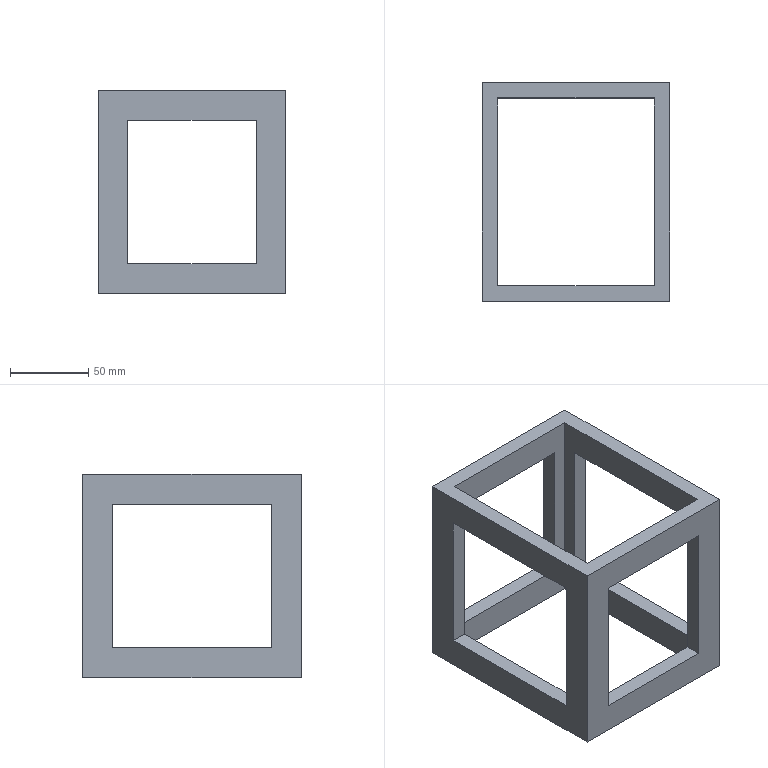Part | SolidWorks | features Cut 2, Extrusion 1 | 1 solid | 26 faces | box 119.912 x 140 x 130 mm | volume 285373 mm3 | plane 26
STEP:
#1=CARTESIAN_POINT('',(-70.,109.,-111.));
#2=VERTEX_POINT('',#1);
#3=CARTESIAN_POINT('',(-70.,109.,-19.));
#4=VERTEX_POINT('',#3);
#5=CARTESIAN_POINT('',(-70.,109.,-111.));
#6=DIRECTION('',(0.,0.,1.));
#7=VECTOR('',#6,1000.);
#8=LINE('',#5,#7);
#9=EDGE_CURVE('',#2,#4,#8,.T.);
#10=ORIENTED_EDGE('',*,*,#9,.F.);
#11=CARTESIAN_POINT('',(-70.,211.,-111.));
#12=VERTEX_POINT('',#11);
#13=CARTESIAN_POINT('',(-70.,211.,-111.));
#14=DIRECTION('',(0.,-1.,0.));
#15=VECTOR('',#14,1000.);
#16=LINE('',#13,#15);
#17=EDGE_CURVE('',#12,#2,#16,.T.);
#18=ORIENTED_EDGE('',*,*,#17,.F.);
#19=CARTESIAN_POINT('',(-70.,211.,-19.));
#20=VERTEX_POINT('',#19);
#21=CARTESIAN_POINT('',(-70.,211.,-19.));
#22=DIRECTION('',(0.,0.,-1.));
#23=VECTOR('',#22,1000.);
#24=LINE('',#21,#23);
#25=EDGE_CURVE('',#20,#12,#24,.T.);
#26=ORIENTED_EDGE('',*,*,#25,.F.);
#27=CARTESIAN_POINT('',(-70.,109.,-19.));
#28=DIRECTION('',(0.,1.,0.));
#29=VECTOR('',#28,1000.);
#30=LINE('',#27,#29);
#31=EDGE_CURVE('',#4,#20,#30,.T.);
#32=ORIENTED_EDGE('',*,*,#31,.F.);
#33=EDGE_LOOP('',(#10,#18,#26,#32));
#34=FACE_BOUND('',#33,.T.);
#35=CARTESIAN_POINT('',(-70.,230.,0.));
#36=VERTEX_POINT('',#35);
#37=CARTESIAN_POINT('',(-70.,90.,0.));
#38=VERTEX_POINT('',#37);
#39=CARTESIAN_POINT('',(-70.,230.,0.));
#40=DIRECTION('',(0.,-1.,0.));
#41=VECTOR('',#40,1000.);
#42=LINE('',#39,#41);
#43=EDGE_CURVE('',#36,#38,#42,.T.);
#44=ORIENTED_EDGE('',*,*,#43,.F.);
#45=CARTESIAN_POINT('',(-70.,230.,-130.));
#46=VERTEX_POINT('',#45);
#47=CARTESIAN_POINT('',(-70.,230.,-130.));
#48=DIRECTION('',(0.,0.,1.));
#49=VECTOR('',#48,1000.);
#50=LINE('',#47,#49);
#51=EDGE_CURVE('',#46,#36,#50,.T.);
#52=ORIENTED_EDGE('',*,*,#51,.F.);
#53=CARTESIAN_POINT('',(-70.,90.,-130.));
#54=VERTEX_POINT('',#53);
#55=CARTESIAN_POINT('',(-70.,230.,-130.));
#56=DIRECTION('',(0.,-1.,0.));
#57=VECTOR('',#56,1000.);
#58=LINE('',#55,#57);
#59=EDGE_CURVE('',#46,#54,#58,.T.);
#60=ORIENTED_EDGE('',*,*,#59,.T.);
#61=CARTESIAN_POINT('',(-70.,90.,-130.));
#62=DIRECTION('',(0.,0.,1.));
#63=VECTOR('',#62,1000.);
#64=LINE('',#61,#63);
#65=EDGE_CURVE('',#54,#38,#64,.T.);
#66=ORIENTED_EDGE('',*,*,#65,.T.);
#67=EDGE_LOOP('',(#44,#52,#60,#66));
#68=FACE_OUTER_BOUND('',#67,.T.);
#69=CARTESIAN_POINT('',(-70.,230.,-130.));
#70=DIRECTION('',(-1.,0.,0.));
#71=DIRECTION('',(0.,-1.,0.));
#72=AXIS2_PLACEMENT_3D('',#69,#70,#71);
#73=PLANE('',#72);
#74=ADVANCED_FACE('',(#34,#68),#73,.T.);
#75=CARTESIAN_POINT('',(30.912,230.,-19.));
#76=VERTEX_POINT('',#75);
#77=CARTESIAN_POINT('',(30.912,230.,-111.));
#78=VERTEX_POINT('',#77);
#79=CARTESIAN_POINT('',(30.912,230.,-130.));
#80=DIRECTION('',(0.,0.,-1.));
#81=VECTOR('',#80,1000.);
#82=LINE('',#79,#81);
#83=EDGE_CURVE('',#76,#78,#82,.T.);
#84=ORIENTED_EDGE('',*,*,#83,.F.);
#85=CARTESIAN_POINT('',(-51.,230.,-19.));
#86=VERTEX_POINT('',#85);
#87=CARTESIAN_POINT('',(49.912,230.,-19.));
#88=DIRECTION('',(1.,0.,0.));
#89=VECTOR('',#88,1000.);
#90=LINE('',#87,#89);
#91=EDGE_CURVE('',#86,#76,#90,.T.);
#92=ORIENTED_EDGE('',*,*,#91,.F.);
#93=CARTESIAN_POINT('',(-51.,230.,-111.));
#94=VERTEX_POINT('',#93);
#95=CARTESIAN_POINT('',(-51.,230.,-130.));
#96=DIRECTION('',(0.,0.,1.));
#97=VECTOR('',#96,1000.);
#98=LINE('',#95,#97);
#99=EDGE_CURVE('',#94,#86,#98,.T.);
#100=ORIENTED_EDGE('',*,*,#99,.F.);
#101=CARTESIAN_POINT('',(49.912,230.,-111.));
#102=DIRECTION('',(-1.,0.,0.));
#103=VECTOR('',#102,1000.);
#104=LINE('',#101,#103);
#105=EDGE_CURVE('',#78,#94,#104,.T.);
#106=ORIENTED_EDGE('',*,*,#105,.F.);
#107=EDGE_LOOP('',(#84,#92,#100,#106));
#108=FACE_BOUND('',#107,.T.);
#109=CARTESIAN_POINT('',(49.912,230.,0.));
#110=VERTEX_POINT('',#109);
#111=CARTESIAN_POINT('',(49.912,230.,0.));
#112=DIRECTION('',(-1.,0.,0.));
#113=VECTOR('',#112,1000.);
#114=LINE('',#111,#113);
#115=EDGE_CURVE('',#110,#36,#114,.T.);
#116=ORIENTED_EDGE('',*,*,#115,.F.);
#117=CARTESIAN_POINT('',(49.912,230.,-130.));
#118=VERTEX_POINT('',#117);
#119=CARTESIAN_POINT('',(49.912,230.,-130.));
#120=DIRECTION('',(0.,0.,1.));
#121=VECTOR('',#120,1000.);
#122=LINE('',#119,#121);
#123=EDGE_CURVE('',#118,#110,#122,.T.);
#124=ORIENTED_EDGE('',*,*,#123,.F.);
#125=CARTESIAN_POINT('',(49.912,230.,-130.));
#126=DIRECTION('',(-1.,0.,0.));
#127=VECTOR('',#126,1000.);
#128=LINE('',#125,#127);
#129=EDGE_CURVE('',#118,#46,#128,.T.);
#130=ORIENTED_EDGE('',*,*,#129,.T.);
#131=ORIENTED_EDGE('',*,*,#51,.T.);
#132=EDGE_LOOP('',(#116,#124,#130,#131));
#133=FACE_OUTER_BOUND('',#132,.T.);
#134=CARTESIAN_POINT('',(49.912,230.,-130.));
#135=DIRECTION('',(0.,1.,0.));
#136=DIRECTION('',(-1.,0.,0.));
#137=AXIS2_PLACEMENT_3D('',#134,#135,#136);
#138=PLANE('',#137);
#139=ADVANCED_FACE('',(#108,#133),#138,.T.);
#140=CARTESIAN_POINT('',(49.912,109.,-19.));
#141=VERTEX_POINT('',#140);
#142=CARTESIAN_POINT('',(49.912,109.,-111.));
#143=VERTEX_POINT('',#142);
#144=CARTESIAN_POINT('',(49.912,109.,-130.));
#145=DIRECTION('',(0.,0.,-1.));
#146=VECTOR('',#145,1000.);
#147=LINE('',#144,#146);
#148=EDGE_CURVE('',#141,#143,#147,.T.);
#149=ORIENTED_EDGE('',*,*,#148,.F.);
#150=CARTESIAN_POINT('',(49.912,211.,-19.));
#151=VERTEX_POINT('',#150);
#152=CARTESIAN_POINT('',(49.912,90.,-19.));
#153=DIRECTION('',(0.,-1.,0.));
#154=VECTOR('',#153,1000.);
#155=LINE('',#152,#154);
#156=EDGE_CURVE('',#151,#141,#155,.T.);
#157=ORIENTED_EDGE('',*,*,#156,.F.);
#158=CARTESIAN_POINT('',(49.912,211.,-111.));
#159=VERTEX_POINT('',#158);
#160=CARTESIAN_POINT('',(49.912,211.,-130.));
#161=DIRECTION('',(0.,0.,1.));
#162=VECTOR('',#161,1000.);
#163=LINE('',#160,#162);
#164=EDGE_CURVE('',#159,#151,#163,.T.);
#165=ORIENTED_EDGE('',*,*,#164,.F.);
#166=CARTESIAN_POINT('',(49.912,90.,-111.));
#167=DIRECTION('',(0.,1.,0.));
#168=VECTOR('',#167,1000.);
#169=LINE('',#166,#168);
#170=EDGE_CURVE('',#143,#159,#169,.T.);
#171=ORIENTED_EDGE('',*,*,#170,.F.);
#172=EDGE_LOOP('',(#149,#157,#165,#171));
#173=FACE_BOUND('',#172,.T.);
#174=CARTESIAN_POINT('',(49.912,90.,0.));
#175=VERTEX_POINT('',#174);
#176=CARTESIAN_POINT('',(49.912,90.,0.));
#177=DIRECTION('',(0.,1.,0.));
#178=VECTOR('',#177,1000.);
#179=LINE('',#176,#178);
#180=EDGE_CURVE('',#175,#110,#179,.T.);
#181=ORIENTED_EDGE('',*,*,#180,.F.);
#182=CARTESIAN_POINT('',(49.912,90.,-130.));
#183=VERTEX_POINT('',#182);
#184=CARTESIAN_POINT('',(49.912,90.,-130.));
#185=DIRECTION('',(0.,0.,1.));
#186=VECTOR('',#185,1000.);
#187=LINE('',#184,#186);
#188=EDGE_CURVE('',#183,#175,#187,.T.);
#189=ORIENTED_EDGE('',*,*,#188,.F.);
#190=CARTESIAN_POINT('',(49.912,90.,-130.));
#191=DIRECTION('',(0.,1.,0.));
#192=VECTOR('',#191,1000.);
#193=LINE('',#190,#192);
#194=EDGE_CURVE('',#183,#118,#193,.T.);
#195=ORIENTED_EDGE('',*,*,#194,.T.);
#196=ORIENTED_EDGE('',*,*,#123,.T.);
#197=EDGE_LOOP('',(#181,#189,#195,#196));
#198=FACE_OUTER_BOUND('',#197,.T.);
#199=CARTESIAN_POINT('',(49.912,90.,-130.));
#200=DIRECTION('',(1.,0.,0.));
#201=DIRECTION('',(0.,0.,-1.));
#202=AXIS2_PLACEMENT_3D('',#199,#200,#201);
#203=PLANE('',#202);
#204=ADVANCED_FACE('',(#173,#198),#203,.T.);
#205=CARTESIAN_POINT('',(30.912,90.,-111.));
#206=VERTEX_POINT('',#205);
#207=CARTESIAN_POINT('',(30.912,90.,-19.));
#208=VERTEX_POINT('',#207);
#209=CARTESIAN_POINT('',(30.912,90.,-111.));
#210=DIRECTION('',(0.,0.,1.));
#211=VECTOR('',#210,1000.);
#212=LINE('',#209,#211);
#213=EDGE_CURVE('',#206,#208,#212,.T.);
#214=ORIENTED_EDGE('',*,*,#213,.F.);
#215=CARTESIAN_POINT('',(-51.,90.,-111.));
#216=VERTEX_POINT('',#215);
#217=CARTESIAN_POINT('',(-51.,90.,-111.));
#218=DIRECTION('',(1.,0.,0.));
#219=VECTOR('',#218,1000.);
#220=LINE('',#217,#219);
#221=EDGE_CURVE('',#216,#206,#220,.T.);
#222=ORIENTED_EDGE('',*,*,#221,.F.);
#223=CARTESIAN_POINT('',(-51.,90.,-19.));
#224=VERTEX_POINT('',#223);
#225=CARTESIAN_POINT('',(-51.,90.,-19.));
#226=DIRECTION('',(0.,0.,-1.));
#227=VECTOR('',#226,1000.);
#228=LINE('',#225,#227);
#229=EDGE_CURVE('',#224,#216,#228,.T.);
#230=ORIENTED_EDGE('',*,*,#229,.F.);
#231=CARTESIAN_POINT('',(30.912,90.,-19.));
#232=DIRECTION('',(-1.,0.,0.));
#233=VECTOR('',#232,1000.);
#234=LINE('',#231,#233);
#235=EDGE_CURVE('',#208,#224,#234,.T.);
#236=ORIENTED_EDGE('',*,*,#235,.F.);
#237=EDGE_LOOP('',(#214,#222,#230,#236));
#238=FACE_BOUND('',#237,.T.);
#239=CARTESIAN_POINT('',(-70.,90.,0.));
#240=DIRECTION('',(1.,0.,0.));
#241=VECTOR('',#240,1000.);
#242=LINE('',#239,#241);
#243=EDGE_CURVE('',#38,#175,#242,.T.);
#244=ORIENTED_EDGE('',*,*,#243,.F.);
#245=ORIENTED_EDGE('',*,*,#65,.F.);
#246=CARTESIAN_POINT('',(-70.,90.,-130.));
#247=DIRECTION('',(1.,0.,0.));
#248=VECTOR('',#247,1000.);
#249=LINE('',#246,#248);
#250=EDGE_CURVE('',#54,#183,#249,.T.);
#251=ORIENTED_EDGE('',*,*,#250,.T.);
#252=ORIENTED_EDGE('',*,*,#188,.T.);
#253=EDGE_LOOP('',(#244,#245,#251,#252));
#254=FACE_OUTER_BOUND('',#253,.T.);
#255=CARTESIAN_POINT('',(-70.,90.,-130.));
#256=DIRECTION('',(0.,-1.,0.));
#257=DIRECTION('',(1.,0.,0.));
#258=AXIS2_PLACEMENT_3D('',#255,#256,#257);
#259=PLANE('',#258);
#260=ADVANCED_FACE('',(#238,#254),#259,.T.);
#261=CARTESIAN_POINT('',(39.912,220.,-130.));
#262=VERTEX_POINT('',#261);
#263=CARTESIAN_POINT('',(-60.,220.,-130.));
#264=VERTEX_POINT('',#263);
#265=CARTESIAN_POINT('',(39.912,220.,-130.));
#266=DIRECTION('',(-1.,0.,0.));
#267=VECTOR('',#266,1000.);
#268=LINE('',#265,#267);
#269=EDGE_CURVE('',#262,#264,#268,.T.);
#270=ORIENTED_EDGE('',*,*,#269,.T.);
#271=CARTESIAN_POINT('',(-60.,100.,-130.));
#272=VERTEX_POINT('',#271);
#273=CARTESIAN_POINT('',(-60.,220.,-130.));
#274=DIRECTION('',(0.,-1.,0.));
#275=VECTOR('',#274,1000.);
#276=LINE('',#273,#275);
#277=EDGE_CURVE('',#264,#272,#276,.T.);
#278=ORIENTED_EDGE('',*,*,#277,.T.);
#279=CARTESIAN_POINT('',(39.912,100.,-130.));
#280=VERTEX_POINT('',#279);
#281=CARTESIAN_POINT('',(-60.,100.,-130.));
#282=DIRECTION('',(1.,0.,0.));
#283=VECTOR('',#282,1000.);
#284=LINE('',#281,#283);
#285=EDGE_CURVE('',#272,#280,#284,.T.);
#286=ORIENTED_EDGE('',*,*,#285,.T.);
#287=CARTESIAN_POINT('',(39.912,100.,-130.));
#288=DIRECTION('',(0.,1.,0.));
#289=VECTOR('',#288,1000.);
#290=LINE('',#287,#289);
#291=EDGE_CURVE('',#280,#262,#290,.T.);
#292=ORIENTED_EDGE('',*,*,#291,.T.);
#293=EDGE_LOOP('',(#270,#278,#286,#292));
#294=FACE_BOUND('',#293,.T.);
#295=ORIENTED_EDGE('',*,*,#59,.F.);
#296=ORIENTED_EDGE('',*,*,#129,.F.);
#297=ORIENTED_EDGE('',*,*,#194,.F.);
#298=ORIENTED_EDGE('',*,*,#250,.F.);
#299=EDGE_LOOP('',(#295,#296,#297,#298));
#300=FACE_OUTER_BOUND('',#299,.T.);
#301=CARTESIAN_POINT('',(0.,0.,-130.));
#302=DIRECTION('',(0.,0.,1.));
#303=DIRECTION('',(1.,0.,0.));
#304=AXIS2_PLACEMENT_3D('',#301,#302,#303);
#305=PLANE('',#304);
#306=ADVANCED_FACE('',(#294,#300),#305,.F.);
#307=CARTESIAN_POINT('',(-60.,220.,0.));
#308=VERTEX_POINT('',#307);
#309=CARTESIAN_POINT('',(-60.,100.,0.));
#310=VERTEX_POINT('',#309);
#311=CARTESIAN_POINT('',(-60.,220.,0.));
#312=DIRECTION('',(0.,-1.,0.));
#313=VECTOR('',#312,1000.);
#314=LINE('',#311,#313);
#315=EDGE_CURVE('',#308,#310,#314,.T.);
#316=ORIENTED_EDGE('',*,*,#315,.F.);
#317=CARTESIAN_POINT('',(39.912,220.,0.));
#318=VERTEX_POINT('',#317);
#319=CARTESIAN_POINT('',(39.912,220.,0.));
#320=DIRECTION('',(-1.,0.,0.));
#321=VECTOR('',#320,1000.);
#322=LINE('',#319,#321);
#323=EDGE_CURVE('',#318,#308,#322,.T.);
#324=ORIENTED_EDGE('',*,*,#323,.F.);
#325=CARTESIAN_POINT('',(39.912,100.,0.));
#326=VERTEX_POINT('',#325);
#327=CARTESIAN_POINT('',(39.912,100.,0.));
#328=DIRECTION('',(0.,1.,0.));
#329=VECTOR('',#328,1000.);
#330=LINE('',#327,#329);
#331=EDGE_CURVE('',#326,#318,#330,.T.);
#332=ORIENTED_EDGE('',*,*,#331,.F.);
#333=CARTESIAN_POINT('',(-60.,100.,0.));
#334=DIRECTION('',(1.,0.,0.));
#335=VECTOR('',#334,1000.);
#336=LINE('',#333,#335);
#337=EDGE_CURVE('',#310,#326,#336,.T.);
#338=ORIENTED_EDGE('',*,*,#337,.F.);
#339=EDGE_LOOP('',(#316,#324,#332,#338));
#340=FACE_BOUND('',#339,.T.);
#341=ORIENTED_EDGE('',*,*,#43,.T.);
#342=ORIENTED_EDGE('',*,*,#243,.T.);
#343=ORIENTED_EDGE('',*,*,#180,.T.);
#344=ORIENTED_EDGE('',*,*,#115,.T.);
#345=EDGE_LOOP('',(#341,#342,#343,#344));
#346=FACE_OUTER_BOUND('',#345,.T.);
#347=CARTESIAN_POINT('',(0.,0.,0.));
#348=DIRECTION('',(0.,0.,1.));
#349=DIRECTION('',(1.,0.,0.));
#350=AXIS2_PLACEMENT_3D('',#347,#348,#349);
#351=PLANE('',#350);
#352=ADVANCED_FACE('',(#340,#346),#351,.T.);
#353=CARTESIAN_POINT('',(-60.,211.,-111.));
#354=VERTEX_POINT('',#353);
#355=CARTESIAN_POINT('',(-60.,109.,-111.));
#356=VERTEX_POINT('',#355);
#357=CARTESIAN_POINT('',(-60.,220.,-111.));
#358=DIRECTION('',(0.,-1.,0.));
#359=VECTOR('',#358,1000.);
#360=LINE('',#357,#359);
#361=EDGE_CURVE('',#354,#356,#360,.T.);
#362=ORIENTED_EDGE('',*,*,#361,.T.);
#363=CARTESIAN_POINT('',(-60.,109.,-19.));
#364=VERTEX_POINT('',#363);
#365=CARTESIAN_POINT('',(-60.,109.,-130.));
#366=DIRECTION('',(0.,0.,1.));
#367=VECTOR('',#366,1000.);
#368=LINE('',#365,#367);
#369=EDGE_CURVE('',#356,#364,#368,.T.);
#370=ORIENTED_EDGE('',*,*,#369,.T.);
#371=CARTESIAN_POINT('',(-60.,211.,-19.));
#372=VERTEX_POINT('',#371);
#373=CARTESIAN_POINT('',(-60.,220.,-19.));
#374=DIRECTION('',(0.,1.,0.));
#375=VECTOR('',#374,1000.);
#376=LINE('',#373,#375);
#377=EDGE_CURVE('',#364,#372,#376,.T.);
#378=ORIENTED_EDGE('',*,*,#377,.T.);
#379=CARTESIAN_POINT('',(-60.,211.,-130.));
#380=DIRECTION('',(0.,0.,-1.));
#381=VECTOR('',#380,1000.);
#382=LINE('',#379,#381);
#383=EDGE_CURVE('',#372,#354,#382,.T.);
#384=ORIENTED_EDGE('',*,*,#383,.T.);
#385=EDGE_LOOP('',(#362,#370,#378,#384));
#386=FACE_BOUND('',#385,.T.);
#387=ORIENTED_EDGE('',*,*,#315,.T.);
#388=CARTESIAN_POINT('',(-60.,100.,-130.));
#389=DIRECTION('',(0.,0.,1.));
#390=VECTOR('',#389,1000.);
#391=LINE('',#388,#390);
#392=EDGE_CURVE('',#272,#310,#391,.T.);
#393=ORIENTED_EDGE('',*,*,#392,.F.);
#394=ORIENTED_EDGE('',*,*,#277,.F.);
#395=CARTESIAN_POINT('',(-60.,220.,-130.));
#396=DIRECTION('',(0.,0.,1.));
#397=VECTOR('',#396,1000.);
#398=LINE('',#395,#397);
#399=EDGE_CURVE('',#264,#308,#398,.T.);
#400=ORIENTED_EDGE('',*,*,#399,.T.);
#401=EDGE_LOOP('',(#387,#393,#394,#400));
#402=FACE_OUTER_BOUND('',#401,.T.);
#403=CARTESIAN_POINT('',(-60.,220.,-130.));
#404=DIRECTION('',(-1.,0.,0.));
#405=DIRECTION('',(0.,-1.,0.));
#406=AXIS2_PLACEMENT_3D('',#403,#404,#405);
#407=PLANE('',#406);
#408=ADVANCED_FACE('',(#386,#402),#407,.F.);
#409=CARTESIAN_POINT('',(-51.,220.,-19.));
#410=VERTEX_POINT('',#409);
#411=CARTESIAN_POINT('',(30.912,220.,-19.));
#412=VERTEX_POINT('',#411);
#413=CARTESIAN_POINT('',(39.912,220.,-19.));
#414=DIRECTION('',(1.,0.,0.));
#415=VECTOR('',#414,1000.);
#416=LINE('',#413,#415);
#417=EDGE_CURVE('',#410,#412,#416,.T.);
#418=ORIENTED_EDGE('',*,*,#417,.T.);
#419=CARTESIAN_POINT('',(30.912,220.,-111.));
#420=VERTEX_POINT('',#419);
#421=CARTESIAN_POINT('',(30.912,220.,-130.));
#422=DIRECTION('',(0.,0.,-1.));
#423=VECTOR('',#422,1000.);
#424=LINE('',#421,#423);
#425=EDGE_CURVE('',#412,#420,#424,.T.);
#426=ORIENTED_EDGE('',*,*,#425,.T.);
#427=CARTESIAN_POINT('',(-51.,220.,-111.));
#428=VERTEX_POINT('',#427);
#429=CARTESIAN_POINT('',(39.912,220.,-111.));
#430=DIRECTION('',(-1.,0.,0.));
#431=VECTOR('',#430,1000.);
#432=LINE('',#429,#431);
#433=EDGE_CURVE('',#420,#428,#432,.T.);
#434=ORIENTED_EDGE('',*,*,#433,.T.);
#435=CARTESIAN_POINT('',(-51.,220.,-130.));
#436=DIRECTION('',(0.,0.,1.));
#437=VECTOR('',#436,1000.);
#438=LINE('',#435,#437);
#439=EDGE_CURVE('',#428,#410,#438,.T.);
#440=ORIENTED_EDGE('',*,*,#439,.T.);
#441=EDGE_LOOP('',(#418,#426,#434,#440));
#442=FACE_BOUND('',#441,.T.);
#443=ORIENTED_EDGE('',*,*,#323,.T.);
#444=ORIENTED_EDGE('',*,*,#399,.F.);
#445=ORIENTED_EDGE('',*,*,#269,.F.);
#446=CARTESIAN_POINT('',(39.912,220.,-130.));
#447=DIRECTION('',(0.,0.,1.));
#448=VECTOR('',#447,1000.);
#449=LINE('',#446,#448);
#450=EDGE_CURVE('',#262,#318,#449,.T.);
#451=ORIENTED_EDGE('',*,*,#450,.T.);
#452=EDGE_LOOP('',(#443,#444,#445,#451));
#453=FACE_OUTER_BOUND('',#452,.T.);
#454=CARTESIAN_POINT('',(39.912,220.,-130.));
#455=DIRECTION('',(0.,1.,0.));
#456=DIRECTION('',(0.,0.,1.));
#457=AXIS2_PLACEMENT_3D('',#454,#455,#456);
#458=PLANE('',#457);
#459=ADVANCED_FACE('',(#442,#453),#458,.F.);
#460=CARTESIAN_POINT('',(39.912,211.,-19.));
#461=VERTEX_POINT('',#460);
#462=CARTESIAN_POINT('',(39.912,109.,-19.));
#463=VERTEX_POINT('',#462);
#464=CARTESIAN_POINT('',(39.912,100.,-19.));
#465=DIRECTION('',(0.,-1.,0.));
#466=VECTOR('',#465,1000.);
#467=LINE('',#464,#466);
#468=EDGE_CURVE('',#461,#463,#467,.T.);
#469=ORIENTED_EDGE('',*,*,#468,.T.);
#470=CARTESIAN_POINT('',(39.912,109.,-111.));
#471=VERTEX_POINT('',#470);
#472=CARTESIAN_POINT('',(39.912,109.,-130.));
#473=DIRECTION('',(0.,0.,-1.));
#474=VECTOR('',#473,1000.);
#475=LINE('',#472,#474);
#476=EDGE_CURVE('',#463,#471,#475,.T.);
#477=ORIENTED_EDGE('',*,*,#476,.T.);
#478=CARTESIAN_POINT('',(39.912,211.,-111.));
#479=VERTEX_POINT('',#478);
#480=CARTESIAN_POINT('',(39.912,100.,-111.));
#481=DIRECTION('',(0.,1.,0.));
#482=VECTOR('',#481,1000.);
#483=LINE('',#480,#482);
#484=EDGE_CURVE('',#471,#479,#483,.T.);
#485=ORIENTED_EDGE('',*,*,#484,.T.);
#486=CARTESIAN_POINT('',(39.912,211.,-130.));
#487=DIRECTION('',(0.,0.,1.));
#488=VECTOR('',#487,1000.);
#489=LINE('',#486,#488);
#490=EDGE_CURVE('',#479,#461,#489,.T.);
#491=ORIENTED_EDGE('',*,*,#490,.T.);
#492=EDGE_LOOP('',(#469,#477,#485,#491));
#493=FACE_BOUND('',#492,.T.);
#494=ORIENTED_EDGE('',*,*,#331,.T.);
#495=ORIENTED_EDGE('',*,*,#450,.F.);
#496=ORIENTED_EDGE('',*,*,#291,.F.);
#497=CARTESIAN_POINT('',(39.912,100.,-130.));
#498=DIRECTION('',(0.,0.,1.));
#499=VECTOR('',#498,1000.);
#500=LINE('',#497,#499);
#501=EDGE_CURVE('',#280,#326,#500,.T.);
#502=ORIENTED_EDGE('',*,*,#501,.T.);
#503=EDGE_LOOP('',(#494,#495,#496,#502));
#504=FACE_OUTER_BOUND('',#503,.T.);
#505=CARTESIAN_POINT('',(39.912,100.,-130.));
#506=DIRECTION('',(1.,0.,0.));
#507=DIRECTION('',(0.,0.,-1.));
#508=AXIS2_PLACEMENT_3D('',#505,#506,#507);
#509=PLANE('',#508);
#510=ADVANCED_FACE('',(#493,#504),#509,.F.);
#511=CARTESIAN_POINT('',(-51.,100.,-111.));
#512=VERTEX_POINT('',#511);
#513=CARTESIAN_POINT('',(30.912,100.,-111.));
#514=VERTEX_POINT('',#513);
#515=CARTESIAN_POINT('',(-60.,100.,-111.));
#516=DIRECTION('',(1.,0.,0.));
#517=VECTOR('',#516,1000.);
#518=LINE('',#515,#517);
#519=EDGE_CURVE('',#512,#514,#518,.T.);
#520=ORIENTED_EDGE('',*,*,#519,.T.);
#521=CARTESIAN_POINT('',(30.912,100.,-19.));
#522=VERTEX_POINT('',#521);
#523=CARTESIAN_POINT('',(30.912,100.,-130.));
#524=DIRECTION('',(0.,0.,1.));
#525=VECTOR('',#524,1000.);
#526=LINE('',#523,#525);
#527=EDGE_CURVE('',#514,#522,#526,.T.);
#528=ORIENTED_EDGE('',*,*,#527,.T.);
#529=CARTESIAN_POINT('',(-51.,100.,-19.));
#530=VERTEX_POINT('',#529);
#531=CARTESIAN_POINT('',(-60.,100.,-19.));
#532=DIRECTION('',(-1.,0.,0.));
#533=VECTOR('',#532,1000.);
#534=LINE('',#531,#533);
#535=EDGE_CURVE('',#522,#530,#534,.T.);
#536=ORIENTED_EDGE('',*,*,#535,.T.);
#537=CARTESIAN_POINT('',(-51.,100.,-130.));
#538=DIRECTION('',(0.,0.,-1.));
#539=VECTOR('',#538,1000.);
#540=LINE('',#537,#539);
#541=EDGE_CURVE('',#530,#512,#540,.T.);
#542=ORIENTED_EDGE('',*,*,#541,.T.);
#543=EDGE_LOOP('',(#520,#528,#536,#542));
#544=FACE_BOUND('',#543,.T.);
#545=ORIENTED_EDGE('',*,*,#337,.T.);
#546=ORIENTED_EDGE('',*,*,#501,.F.);
#547=ORIENTED_EDGE('',*,*,#285,.F.);
#548=ORIENTED_EDGE('',*,*,#392,.T.);
#549=EDGE_LOOP('',(#545,#546,#547,#548));
#550=FACE_OUTER_BOUND('',#549,.T.);
#551=CARTESIAN_POINT('',(-60.,100.,-130.));
#552=DIRECTION('',(0.,-1.,0.));
#553=DIRECTION('',(0.,0.,-1.));
#554=AXIS2_PLACEMENT_3D('',#551,#552,#553);
#555=PLANE('',#554);
#556=ADVANCED_FACE('',(#544,#550),#555,.F.);
#557=CARTESIAN_POINT('',(30.912,348.,-19.));
#558=DIRECTION('',(0.,-1.,0.));
#559=VECTOR('',#558,1000.);
#560=LINE('',#557,#559);
#561=EDGE_CURVE('',#522,#208,#560,.T.);
#562=ORIENTED_EDGE('',*,*,#561,.T.);
#563=ORIENTED_EDGE('',*,*,#235,.T.);
#564=CARTESIAN_POINT('',(-51.,348.,-19.));
#565=DIRECTION('',(0.,-1.,0.));
#566=VECTOR('',#565,1000.);
#567=LINE('',#564,#566);
#568=EDGE_CURVE('',#530,#224,#567,.T.);
#569=ORIENTED_EDGE('',*,*,#568,.F.);
#570=ORIENTED_EDGE('',*,*,#535,.F.);
#571=EDGE_LOOP('',(#562,#563,#569,#570));
#572=FACE_OUTER_BOUND('',#571,.T.);
#573=CARTESIAN_POINT('',(30.912,348.,-19.));
#574=DIRECTION('',(0.,0.,1.));
#575=DIRECTION('',(1.,0.,0.));
#576=AXIS2_PLACEMENT_3D('',#573,#574,#575);
#577=PLANE('',#576);
#578=ADVANCED_FACE('',(#572),#577,.F.);
#579=ORIENTED_EDGE('',*,*,#568,.T.);
#580=ORIENTED_EDGE('',*,*,#229,.T.);
#581=CARTESIAN_POINT('',(-51.,348.,-111.));
#582=DIRECTION('',(0.,-1.,0.));
#583=VECTOR('',#582,1000.);
#584=LINE('',#581,#583);
#585=EDGE_CURVE('',#512,#216,#584,.T.);
#586=ORIENTED_EDGE('',*,*,#585,.F.);
#587=ORIENTED_EDGE('',*,*,#541,.F.);
#588=EDGE_LOOP('',(#579,#580,#586,#587));
#589=FACE_OUTER_BOUND('',#588,.T.);
#590=CARTESIAN_POINT('',(-51.,348.,-19.));
#591=DIRECTION('',(-1.,0.,0.));
#592=DIRECTION('',(0.,-1.,0.));
#593=AXIS2_PLACEMENT_3D('',#590,#591,#592);
#594=PLANE('',#593);
#595=ADVANCED_FACE('',(#589),#594,.F.);
#596=ORIENTED_EDGE('',*,*,#585,.T.);
#597=ORIENTED_EDGE('',*,*,#221,.T.);
#598=CARTESIAN_POINT('',(30.912,348.,-111.));
#599=DIRECTION('',(0.,-1.,0.));
#600=VECTOR('',#599,1000.);
#601=LINE('',#598,#600);
#602=EDGE_CURVE('',#514,#206,#601,.T.);
#603=ORIENTED_EDGE('',*,*,#602,.F.);
#604=ORIENTED_EDGE('',*,*,#519,.F.);
#605=EDGE_LOOP('',(#596,#597,#603,#604));
#606=FACE_OUTER_BOUND('',#605,.T.);
#607=CARTESIAN_POINT('',(-51.,348.,-111.));
#608=DIRECTION('',(0.,0.,-1.));
#609=DIRECTION('',(-1.,0.,0.));
#610=AXIS2_PLACEMENT_3D('',#607,#608,#609);
#611=PLANE('',#610);
#612=ADVANCED_FACE('',(#606),#611,.F.);
#613=ORIENTED_EDGE('',*,*,#602,.T.);
#614=ORIENTED_EDGE('',*,*,#213,.T.);
#615=ORIENTED_EDGE('',*,*,#561,.F.);
#616=ORIENTED_EDGE('',*,*,#527,.F.);
#617=EDGE_LOOP('',(#613,#614,#615,#616));
#618=FACE_OUTER_BOUND('',#617,.T.);
#619=CARTESIAN_POINT('',(30.912,348.,-111.));
#620=DIRECTION('',(1.,0.,0.));
#621=DIRECTION('',(0.,1.,0.));
#622=AXIS2_PLACEMENT_3D('',#619,#620,#621);
#623=PLANE('',#622);
#624=ADVANCED_FACE('',(#618),#623,.F.);
#625=ORIENTED_EDGE('',*,*,#83,.T.);
#626=CARTESIAN_POINT('',(30.912,348.,-111.));
#627=DIRECTION('',(0.,-1.,0.));
#628=VECTOR('',#627,1000.);
#629=LINE('',#626,#628);
#630=EDGE_CURVE('',#78,#420,#629,.T.);
#631=ORIENTED_EDGE('',*,*,#630,.T.);
#632=ORIENTED_EDGE('',*,*,#425,.F.);
#633=CARTESIAN_POINT('',(30.912,348.,-19.));
#634=DIRECTION('',(0.,-1.,0.));
#635=VECTOR('',#634,1000.);
#636=LINE('',#633,#635);
#637=EDGE_CURVE('',#76,#412,#636,.T.);
#638=ORIENTED_EDGE('',*,*,#637,.F.);
#639=EDGE_LOOP('',(#625,#631,#632,#638));
#640=FACE_OUTER_BOUND('',#639,.T.);
#641=CARTESIAN_POINT('',(30.912,348.,-111.));
#642=DIRECTION('',(1.,0.,0.));
#643=DIRECTION('',(0.,1.,0.));
#644=AXIS2_PLACEMENT_3D('',#641,#642,#643);
#645=PLANE('',#644);
#646=ADVANCED_FACE('',(#640),#645,.F.);
#647=ORIENTED_EDGE('',*,*,#105,.T.);
#648=CARTESIAN_POINT('',(-51.,348.,-111.));
#649=DIRECTION('',(0.,-1.,0.));
#650=VECTOR('',#649,1000.);
#651=LINE('',#648,#650);
#652=EDGE_CURVE('',#94,#428,#651,.T.);
#653=ORIENTED_EDGE('',*,*,#652,.T.);
#654=ORIENTED_EDGE('',*,*,#433,.F.);
#655=ORIENTED_EDGE('',*,*,#630,.F.);
#656=EDGE_LOOP('',(#647,#653,#654,#655));
#657=FACE_OUTER_BOUND('',#656,.T.);
#658=CARTESIAN_POINT('',(-51.,348.,-111.));
#659=DIRECTION('',(0.,0.,-1.));
#660=DIRECTION('',(-1.,0.,0.));
#661=AXIS2_PLACEMENT_3D('',#658,#659,#660);
#662=PLANE('',#661);
#663=ADVANCED_FACE('',(#657),#662,.F.);
#664=ORIENTED_EDGE('',*,*,#99,.T.);
#665=CARTESIAN_POINT('',(-51.,348.,-19.));
#666=DIRECTION('',(0.,-1.,0.));
#667=VECTOR('',#666,1000.);
#668=LINE('',#665,#667);
#669=EDGE_CURVE('',#86,#410,#668,.T.);
#670=ORIENTED_EDGE('',*,*,#669,.T.);
#671=ORIENTED_EDGE('',*,*,#439,.F.);
#672=ORIENTED_EDGE('',*,*,#652,.F.);
#673=EDGE_LOOP('',(#664,#670,#671,#672));
#674=FACE_OUTER_BOUND('',#673,.T.);
#675=CARTESIAN_POINT('',(-51.,348.,-19.));
#676=DIRECTION('',(-1.,0.,0.));
#677=DIRECTION('',(0.,-1.,0.));
#678=AXIS2_PLACEMENT_3D('',#675,#676,#677);
#679=PLANE('',#678);
#680=ADVANCED_FACE('',(#674),#679,.F.);
#681=ORIENTED_EDGE('',*,*,#91,.T.);
#682=ORIENTED_EDGE('',*,*,#637,.T.);
#683=ORIENTED_EDGE('',*,*,#417,.F.);
#684=ORIENTED_EDGE('',*,*,#669,.F.);
#685=EDGE_LOOP('',(#681,#682,#683,#684));
#686=FACE_OUTER_BOUND('',#685,.T.);
#687=CARTESIAN_POINT('',(30.912,348.,-19.));
#688=DIRECTION('',(0.,0.,1.));
#689=DIRECTION('',(1.,0.,0.));
#690=AXIS2_PLACEMENT_3D('',#687,#688,#689);
#691=PLANE('',#690);
#692=ADVANCED_FACE('',(#686),#691,.F.);
#693=ORIENTED_EDGE('',*,*,#156,.T.);
#694=CARTESIAN_POINT('',(188.,109.,-19.));
#695=DIRECTION('',(-1.,0.,0.));
#696=VECTOR('',#695,1000.);
#697=LINE('',#694,#696);
#698=EDGE_CURVE('',#141,#463,#697,.T.);
#699=ORIENTED_EDGE('',*,*,#698,.T.);
#700=ORIENTED_EDGE('',*,*,#468,.F.);
#701=CARTESIAN_POINT('',(188.,211.,-19.));
#702=DIRECTION('',(-1.,0.,0.));
#703=VECTOR('',#702,1000.);
#704=LINE('',#701,#703);
#705=EDGE_CURVE('',#151,#461,#704,.T.);
#706=ORIENTED_EDGE('',*,*,#705,.F.);
#707=EDGE_LOOP('',(#693,#699,#700,#706));
#708=FACE_OUTER_BOUND('',#707,.T.);
#709=CARTESIAN_POINT('',(188.,109.,-19.));
#710=DIRECTION('',(0.,0.,1.));
#711=DIRECTION('',(1.,0.,0.));
#712=AXIS2_PLACEMENT_3D('',#709,#710,#711);
#713=PLANE('',#712);
#714=ADVANCED_FACE('',(#708),#713,.F.);
#715=ORIENTED_EDGE('',*,*,#164,.T.);
#716=ORIENTED_EDGE('',*,*,#705,.T.);
#717=ORIENTED_EDGE('',*,*,#490,.F.);
#718=CARTESIAN_POINT('',(188.,211.,-111.));
#719=DIRECTION('',(-1.,0.,0.));
#720=VECTOR('',#719,1000.);
#721=LINE('',#718,#720);
#722=EDGE_CURVE('',#159,#479,#721,.T.);
#723=ORIENTED_EDGE('',*,*,#722,.F.);
#724=EDGE_LOOP('',(#715,#716,#717,#723));
#725=FACE_OUTER_BOUND('',#724,.T.);
#726=CARTESIAN_POINT('',(188.,211.,-19.));
#727=DIRECTION('',(0.,1.,0.));
#728=DIRECTION('',(-1.,0.,0.));
#729=AXIS2_PLACEMENT_3D('',#726,#727,#728);
#730=PLANE('',#729);
#731=ADVANCED_FACE('',(#725),#730,.F.);
#732=ORIENTED_EDGE('',*,*,#170,.T.);
#733=ORIENTED_EDGE('',*,*,#722,.T.);
#734=ORIENTED_EDGE('',*,*,#484,.F.);
#735=CARTESIAN_POINT('',(188.,109.,-111.));
#736=DIRECTION('',(-1.,0.,0.));
#737=VECTOR('',#736,1000.);
#738=LINE('',#735,#737);
#739=EDGE_CURVE('',#143,#471,#738,.T.);
#740=ORIENTED_EDGE('',*,*,#739,.F.);
#741=EDGE_LOOP('',(#732,#733,#734,#740));
#742=FACE_OUTER_BOUND('',#741,.T.);
#743=CARTESIAN_POINT('',(188.,211.,-111.));
#744=DIRECTION('',(0.,0.,-1.));
#745=DIRECTION('',(-1.,0.,0.));
#746=AXIS2_PLACEMENT_3D('',#743,#744,#745);
#747=PLANE('',#746);
#748=ADVANCED_FACE('',(#742),#747,.F.);
#749=ORIENTED_EDGE('',*,*,#148,.T.);
#750=ORIENTED_EDGE('',*,*,#739,.T.);
#751=ORIENTED_EDGE('',*,*,#476,.F.);
#752=ORIENTED_EDGE('',*,*,#698,.F.);
#753=EDGE_LOOP('',(#749,#750,#751,#752));
#754=FACE_OUTER_BOUND('',#753,.T.);
#755=CARTESIAN_POINT('',(188.,109.,-111.));
#756=DIRECTION('',(0.,-1.,0.));
#757=DIRECTION('',(1.,0.,0.));
#758=AXIS2_PLACEMENT_3D('',#755,#756,#757);
#759=PLANE('',#758);
#760=ADVANCED_FACE('',(#754),#759,.F.);
#761=CARTESIAN_POINT('',(188.,109.,-111.));
#762=DIRECTION('',(-1.,0.,0.));
#763=VECTOR('',#762,1000.);
#764=LINE('',#761,#763);
#765=EDGE_CURVE('',#356,#2,#764,.T.);
#766=ORIENTED_EDGE('',*,*,#765,.T.);
#767=ORIENTED_EDGE('',*,*,#9,.T.);
#768=CARTESIAN_POINT('',(188.,109.,-19.));
#769=DIRECTION('',(-1.,0.,0.));
#770=VECTOR('',#769,1000.);
#771=LINE('',#768,#770);
#772=EDGE_CURVE('',#364,#4,#771,.T.);
#773=ORIENTED_EDGE('',*,*,#772,.F.);
#774=ORIENTED_EDGE('',*,*,#369,.F.);
#775=EDGE_LOOP('',(#766,#767,#773,#774));
#776=FACE_OUTER_BOUND('',#775,.T.);
#777=CARTESIAN_POINT('',(188.,109.,-111.));
#778=DIRECTION('',(0.,-1.,0.));
#779=DIRECTION('',(1.,0.,0.));
#780=AXIS2_PLACEMENT_3D('',#777,#778,#779);
#781=PLANE('',#780);
#782=ADVANCED_FACE('',(#776),#781,.F.);
#783=CARTESIAN_POINT('',(188.,211.,-111.));
#784=DIRECTION('',(-1.,0.,0.));
#785=VECTOR('',#784,1000.);
#786=LINE('',#783,#785);
#787=EDGE_CURVE('',#354,#12,#786,.T.);
#788=ORIENTED_EDGE('',*,*,#787,.T.);
#789=ORIENTED_EDGE('',*,*,#17,.T.);
#790=ORIENTED_EDGE('',*,*,#765,.F.);
#791=ORIENTED_EDGE('',*,*,#361,.F.);
#792=EDGE_LOOP('',(#788,#789,#790,#791));
#793=FACE_OUTER_BOUND('',#792,.T.);
#794=CARTESIAN_POINT('',(188.,211.,-111.));
#795=DIRECTION('',(0.,0.,-1.));
#796=DIRECTION('',(-1.,0.,0.));
#797=AXIS2_PLACEMENT_3D('',#794,#795,#796);
#798=PLANE('',#797);
#799=ADVANCED_FACE('',(#793),#798,.F.);
#800=CARTESIAN_POINT('',(188.,211.,-19.));
#801=DIRECTION('',(-1.,0.,0.));
#802=VECTOR('',#801,1000.);
#803=LINE('',#800,#802);
#804=EDGE_CURVE('',#372,#20,#803,.T.);
#805=ORIENTED_EDGE('',*,*,#804,.T.);
#806=ORIENTED_EDGE('',*,*,#25,.T.);
#807=ORIENTED_EDGE('',*,*,#787,.F.);
#808=ORIENTED_EDGE('',*,*,#383,.F.);
#809=EDGE_LOOP('',(#805,#806,#807,#808));
#810=FACE_OUTER_BOUND('',#809,.T.);
#811=CARTESIAN_POINT('',(188.,211.,-19.));
#812=DIRECTION('',(0.,1.,0.));
#813=DIRECTION('',(-1.,0.,0.));
#814=AXIS2_PLACEMENT_3D('',#811,#812,#813);
#815=PLANE('',#814);
#816=ADVANCED_FACE('',(#810),#815,.F.);
#817=ORIENTED_EDGE('',*,*,#772,.T.);
#818=ORIENTED_EDGE('',*,*,#31,.T.);
#819=ORIENTED_EDGE('',*,*,#804,.F.);
#820=ORIENTED_EDGE('',*,*,#377,.F.);
#821=EDGE_LOOP('',(#817,#818,#819,#820));
#822=FACE_OUTER_BOUND('',#821,.T.);
#823=CARTESIAN_POINT('',(188.,109.,-19.));
#824=DIRECTION('',(0.,0.,1.));
#825=DIRECTION('',(1.,0.,0.));
#826=AXIS2_PLACEMENT_3D('',#823,#824,#825);
#827=PLANE('',#826);
#828=ADVANCED_FACE('',(#822),#827,.F.);
#829=CLOSED_SHELL('',(#74,#139,#204,#260,#306,#352,#408,#459,#510,#556,#578,#595,#612,#624,#646,#663,#680,#692,#714,#731,#748,#760,#782,#799,#816,#828));
#830=MANIFOLD_SOLID_BREP('',#829);
#831=CARTESIAN_POINT('',(0.,0.,0.));
#832=DIRECTION('',(0.,0.,1.));
#833=DIRECTION('',(1.,0.,0.));
#834=AXIS2_PLACEMENT_3D('',#831,#832,#833);
#835=(LENGTH_UNIT()NAMED_UNIT(*)SI_UNIT(.MILLI.,.METRE.));
#836=UNCERTAINTY_MEASURE_WITH_UNIT(LENGTH_MEASURE(0.00001),#835,'','');
#837=(NAMED_UNIT(*)PLANE_ANGLE_UNIT()SI_UNIT($,.RADIAN.));
#838=(NAMED_UNIT(*)SI_UNIT($,.STERADIAN.)SOLID_ANGLE_UNIT());
#839=(GEOMETRIC_REPRESENTATION_CONTEXT(3)GLOBAL_UNCERTAINTY_ASSIGNED_CONTEXT((#836))GLOBAL_UNIT_ASSIGNED_CONTEXT((#835,#837,#838))REPRESENTATION_CONTEXT('',''));
#840=ADVANCED_BREP_SHAPE_REPRESENTATION('',(#830,#834),#839);